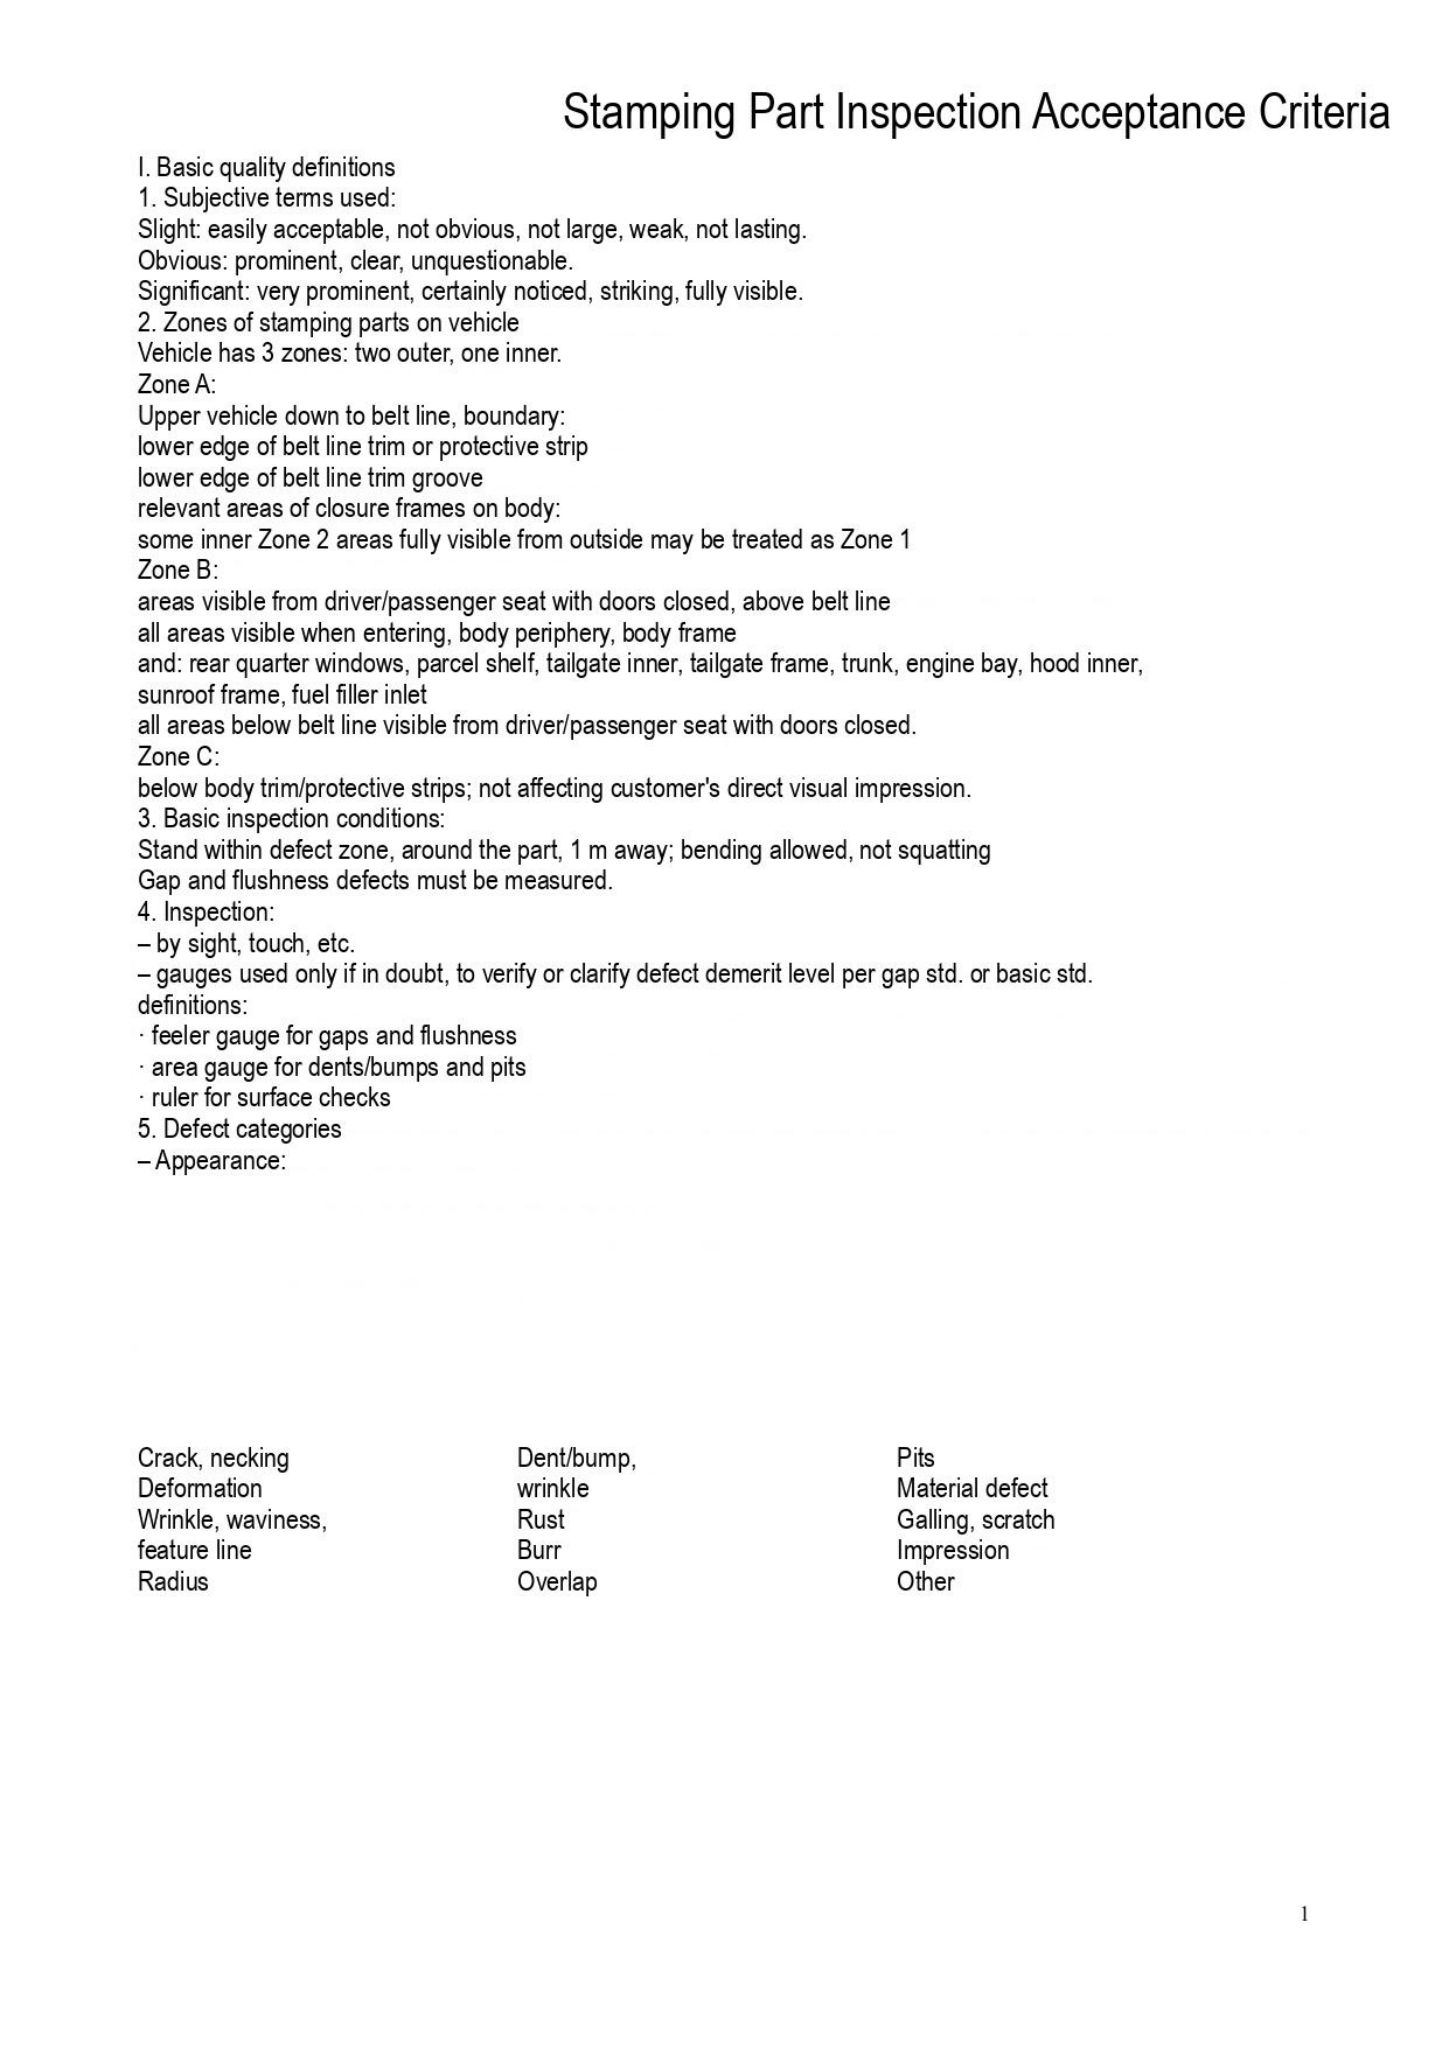Stamping Part Inspection Acceptance Criteria

I. Basic quality definitions
1. Subjective terms used:
Slight: easily acceptable, not obvious, not large, weak, not lasting.
Obvious: prominent, clear, unquestionable.
Significant: very prominent, certainly noticed, striking, fully visible.
2. Zones of stamping parts on vehicle
Vehicle has 3 zones: two outer, one inner.
Zone A:
Upper vehicle down to belt line, boundary:
lower edge of belt line trim or protective strip
lower edge of belt line trim groove
relevant areas of closure frames on body:
some inner Zone 2 areas fully visible from outside may be treated as Zone 1
Zone B:
areas visible from driver/passenger seat with doors closed, above belt line
all areas visible when entering, body periphery, body frame
and: rear quarter windows, parcel shelf, tailgate inner, tailgate frame, trunk, engine bay, hood inner, sunroof frame, fuel filler inlet
all areas below belt line visible from driver/passenger seat with doors closed.
Zone C:
below body trim/protective strips; not affecting customer's direct visual impression.
3. Basic inspection conditions:
Stand within defect zone, around the part, 1 m away; bending allowed, not squatting
Gap and flushness defects must be measured.
4. Inspection:
– by sight, touch, etc.
– gauges used only if in doubt, to verify or clarify defect demerit level per gap std. or basic std.
definitions:
· feeler gauge for gaps and flushness
· area gauge for dents/bumps and pits
· ruler for surface checks
5. Defect categories
– Appearance:

| | | |
|---|---|---|
| Crack, necking | Dent/bump, wrinkle | Pits |
| Deformation | Rust | Material defect |
| Wrinkle, waviness, feature line | Burr | Galling, scratch |
| Radius | Overlap | Impression |
| | | Other |

1
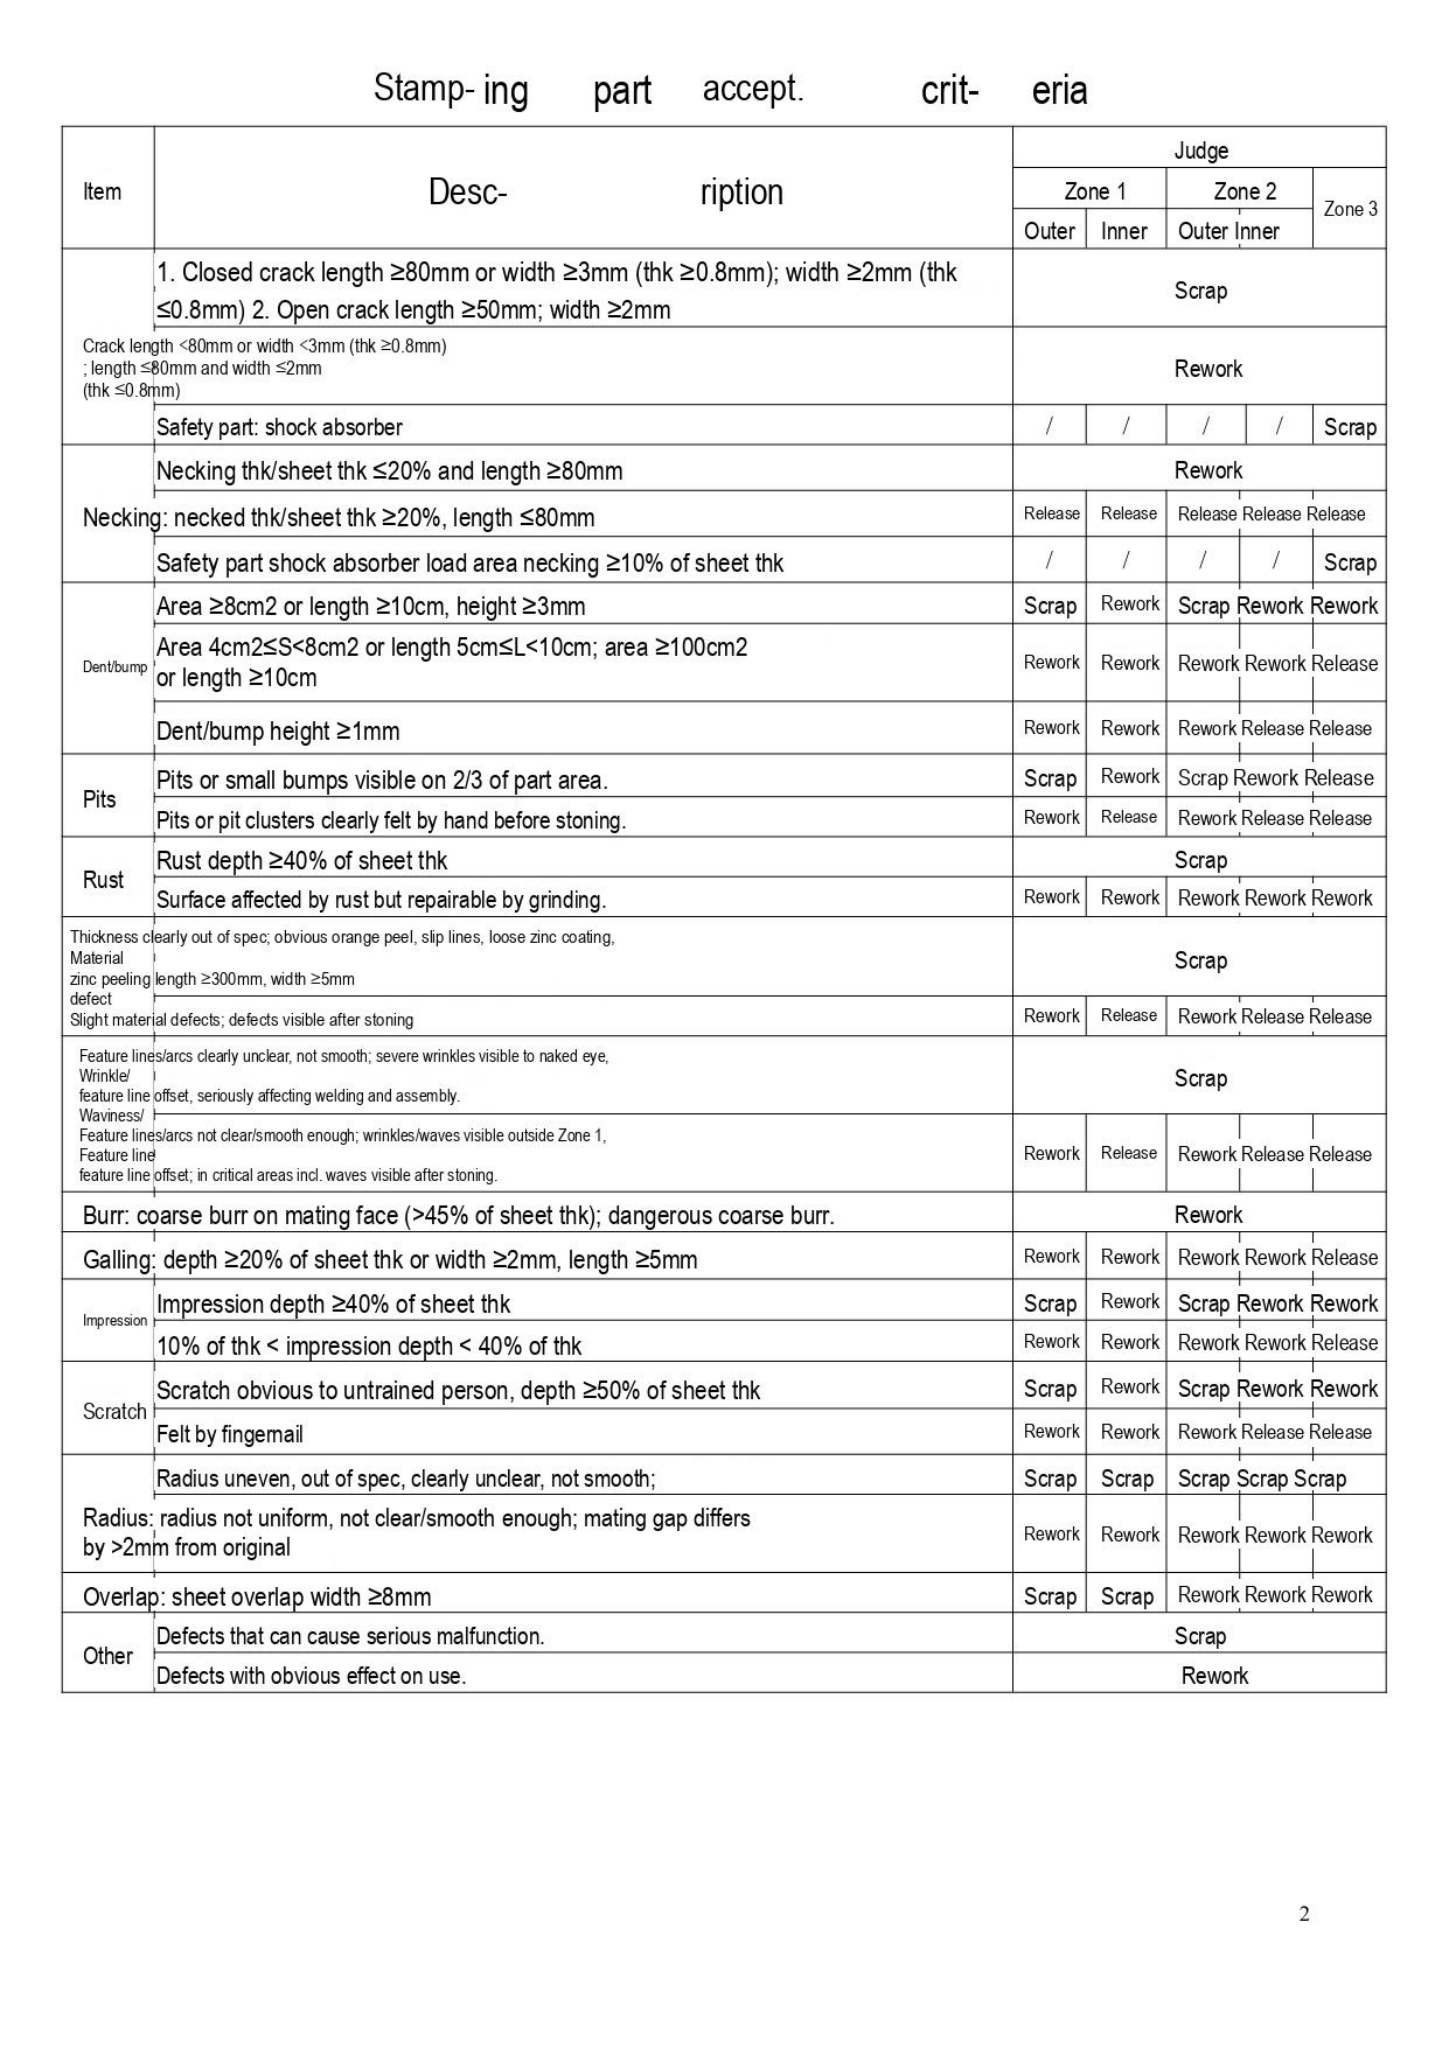Stamp- ing part accept. crit- eria

| Item | Description | Zone 1 Outer | Zone 1 Inner | Zone 2 Outer | Zone 2 Inner | Zone 3 |
|---|---|---|---|---|---|---|
| Crack | 1. Closed crack length ≥80mm or width ≥3mm (thk ≥0.8mm); width ≥2mm (thk ≤0.8mm) 2. Open crack length ≥50mm; width ≥2mm | Scrap | | | | |
| | Crack length <80mm or width <3mm (thk ≥0.8mm); length ≤80mm and width ≤2mm (thk ≤0.8mm) | Rework | | | | |
| | Safety part: shock absorber | / | / | / | / | Scrap |
| Necking | Necking thk/sheet thk ≤20% and length ≥80mm | Rework | | | | |
| | necked thk/sheet thk ≥20%, length ≤80mm | Release | Release | Release | Release | Release |
| | Safety part shock absorber load area necking ≥10% of sheet thk | / | / | / | / | Scrap |
| Dent/bump | Area ≥8cm2 or length ≥10cm, height ≥3mm | Scrap | Rework | Scrap | Rework | Rework |
| | Area 4cm2≤S<8cm2 or length 5cm≤L<10cm; area ≥100cm2 or length ≥10cm | Rework | Rework | Rework | Rework | Release |
| | Dent/bump height ≥1mm | Rework | Rework | Rework | Release | Release |
| Pits | Pits or small bumps visible on 2/3 of part area. | Scrap | Rework | Scrap | Rework | Release |
| | Pits or pit clusters clearly felt by hand before stoning. | Rework | Release | Rework | Release | Release |
| Rust | Rust depth ≥40% of sheet thk | Scrap | | | | |
| | Surface affected by rust but repairable by grinding. | Rework | Rework | Rework | Rework | Rework |
| Material defect | Thickness clearly out of spec; obvious orange peel, slip lines, loose zinc coating, zinc peeling length ≥300mm, width ≥5mm | Scrap | | | | |
| | Slight material defects; defects visible after stoning | Rework | Release | Rework | Release | Release |
| Wrinkle/ Waviness/ Feature line | Feature lines/arcs clearly unclear, not smooth; severe wrinkles visible to naked eye, feature line offset, seriously affecting welding and assembly. | Scrap | | | | |
| | Feature lines/arcs not clear/smooth enough; wrinkles/waves visible outside Zone 1, feature line offset; in critical areas incl. waves visible after stoning. | Rework | Release | Rework | Release | Release |
| Burr | coarse burr on mating face (>45% of sheet thk); dangerous coarse burr. | Rework | | | | |
| Galling | depth ≥20% of sheet thk or width ≥2mm, length ≥5mm | Rework | Rework | Rework | Rework | Release |
| Impression | Impression depth ≥40% of sheet thk | Scrap | Rework | Scrap | Rework | Rework |
| | 10% of thk < impression depth < 40% of thk | Rework | Rework | Rework | Rework | Release |
| Scratch | Scratch obvious to untrained person, depth ≥50% of sheet thk | Scrap | Rework | Scrap | Rework | Rework |
| | Felt by fingernail | Rework | Rework | Rework | Release | Release |
| Radius | Radius uneven, out of spec, clearly unclear, not smooth; | Scrap | Scrap | Scrap | Scrap | Scrap |
| | radius not uniform, not clear/smooth enough; mating gap differs by >2mm from original | Rework | Rework | Rework | Rework | Rework |
| Overlap | sheet overlap width ≥8mm | Scrap | Scrap | Rework | Rework | Rework |
| Other | Defects that can cause serious malfunction. | Scrap | | | | |
| | Defects with obvious effect on use. | Rework | | | | |

2
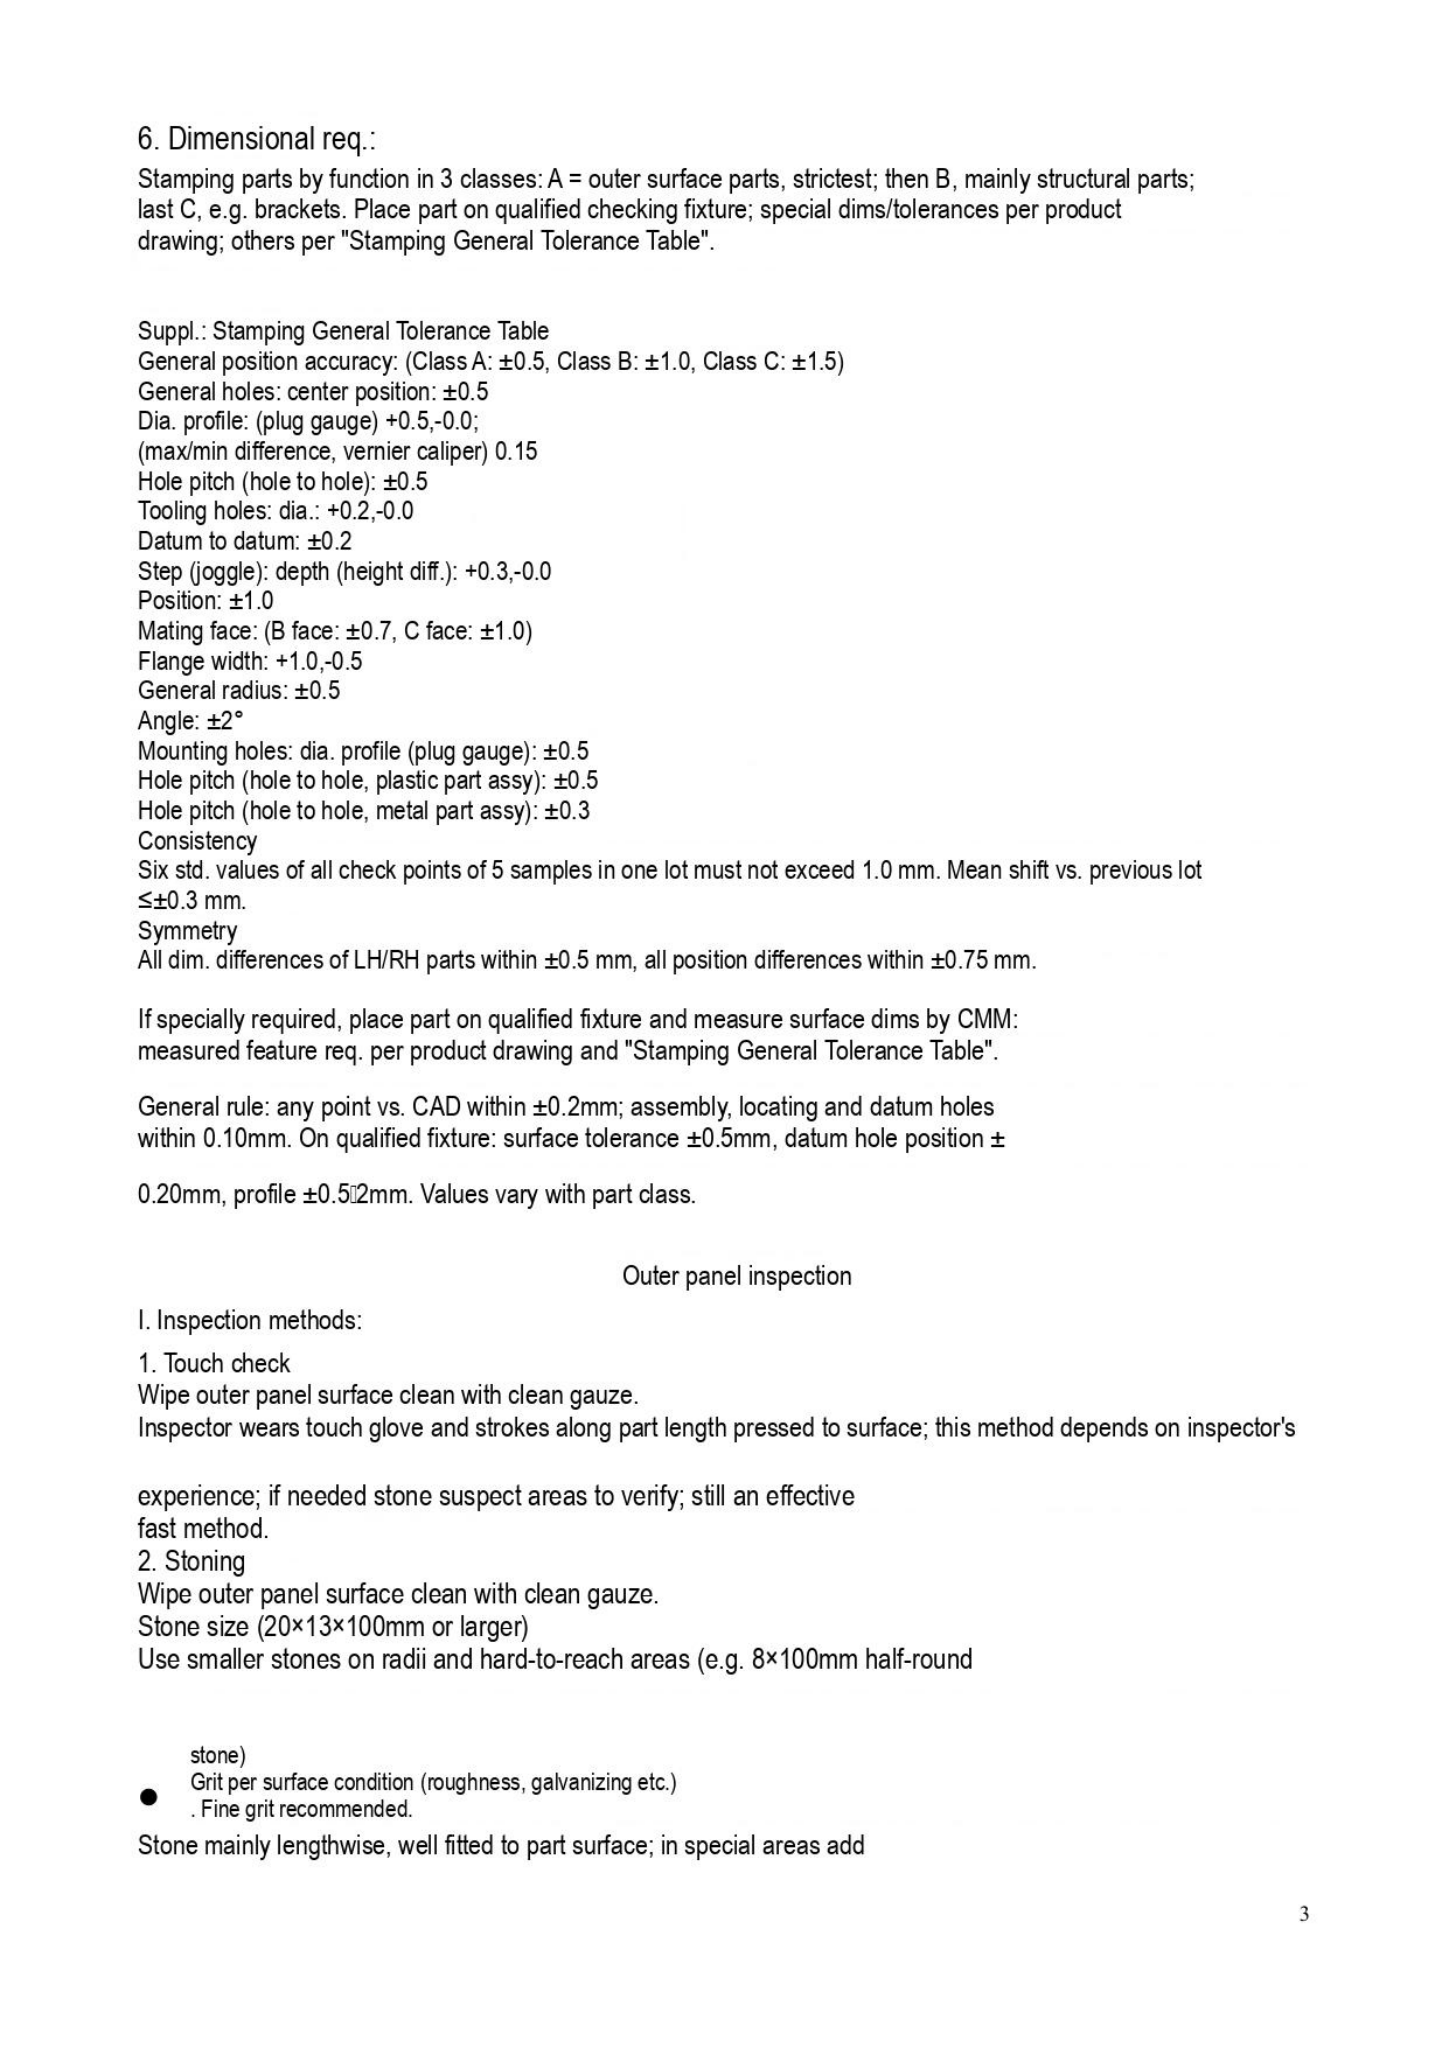6. Dimensional req.:
Stamping parts by function in 3 classes: A = outer surface parts, strictest; then B, mainly structural parts; last C, e.g. brackets. Place part on qualified checking fixture; special dims/tolerances per product drawing; others per "Stamping General Tolerance Table".

Suppl.: Stamping General Tolerance Table
General position accuracy: (Class A: ±0.5, Class B: ±1.0, Class C: ±1.5)
General holes: center position: ±0.5
Dia. profile: (plug gauge) +0.5,-0.0;
(max/min difference, vernier caliper) 0.15
Hole pitch (hole to hole): ±0.5
Tooling holes: dia.: +0.2,-0.0
Datum to datum: ±0.2
Step (joggle): depth (height diff.): +0.3,-0.0
Position: ±1.0
Mating face: (B face: ±0.7, C face: ±1.0)
Flange width: +1.0,-0.5
General radius: ±0.5
Angle: ±2°
Mounting holes: dia. profile (plug gauge): ±0.5
Hole pitch (hole to hole, plastic part assy): ±0.5
Hole pitch (hole to hole, metal part assy): ±0.3
Consistency
Six std. values of all check points of 5 samples in one lot must not exceed 1.0 mm. Mean shift vs. previous lot ≤±0.3 mm.
Symmetry
All dim. differences of LH/RH parts within ±0.5 mm, all position differences within ±0.75 mm.

If specially required, place part on qualified fixture and measure surface dims by CMM: measured feature req. per product drawing and "Stamping General Tolerance Table".

General rule: any point vs. CAD within ±0.2mm; assembly, locating and datum holes within 0.10mm. On qualified fixture: surface tolerance ±0.5mm, datum hole position ±

0.20mm, profile ±0.5 2mm. Values vary with part class.

Outer panel inspection

I. Inspection methods:

1. Touch check
Wipe outer panel surface clean with clean gauze.
Inspector wears touch glove and strokes along part length pressed to surface; this method depends on inspector's

experience; if needed stone suspect areas to verify; still an effective fast method.
2. Stoning
Wipe outer panel surface clean with clean gauze.
Stone size (20×13×100mm or larger)
Use smaller stones on radii and hard-to-reach areas (e.g. 8×100mm half-round

stone)
- Grit per surface condition (roughness, galvanizing etc.)
. Fine grit recommended.

Stone mainly lengthwise, well fitted to part surface; in special areas add

3
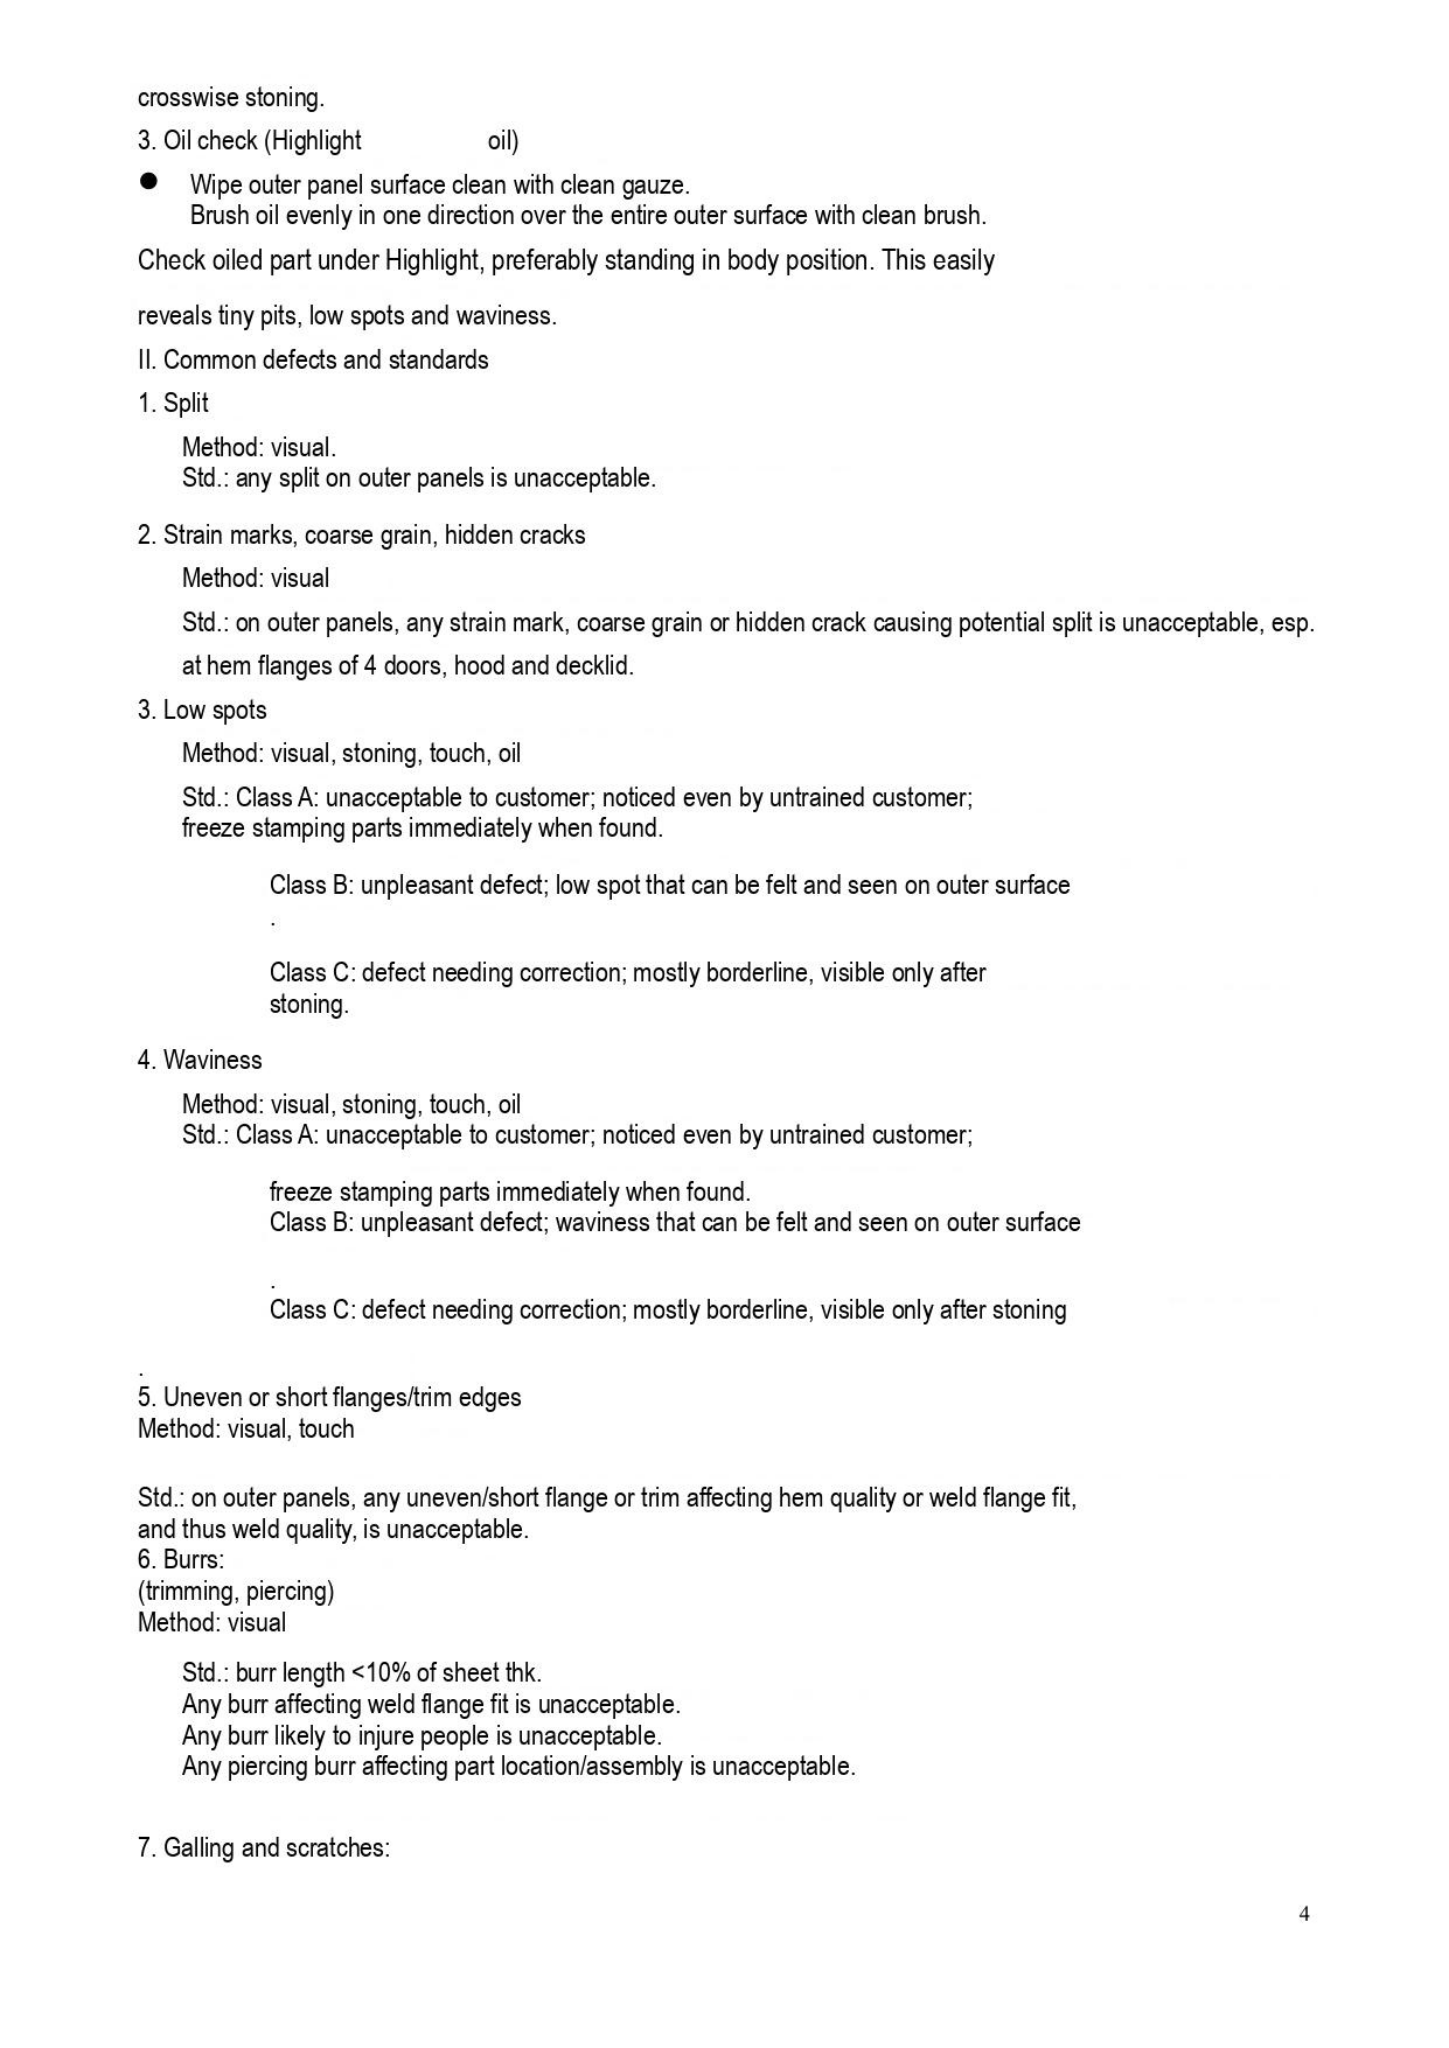crosswise stoning.

3. Oil check (Highlight oil)

● Wipe outer panel surface clean with clean gauze.
Brush oil evenly in one direction over the entire outer surface with clean brush.

Check oiled part under Highlight, preferably standing in body position. This easily

reveals tiny pits, low spots and waviness.

II. Common defects and standards

1. Split

Method: visual.
Std.: any split on outer panels is unacceptable.

2. Strain marks, coarse grain, hidden cracks

Method: visual

Std.: on outer panels, any strain mark, coarse grain or hidden crack causing potential split is unacceptable, esp. at hem flanges of 4 doors, hood and decklid.

3. Low spots

Method: visual, stoning, touch, oil

Std.: Class A: unacceptable to customer; noticed even by untrained customer; freeze stamping parts immediately when found.

Class B: unpleasant defect; low spot that can be felt and seen on outer surface
.

Class C: defect needing correction; mostly borderline, visible only after stoning.

4. Waviness

Method: visual, stoning, touch, oil
Std.: Class A: unacceptable to customer; noticed even by untrained customer;

freeze stamping parts immediately when found.
Class B: unpleasant defect; waviness that can be felt and seen on outer surface

.
Class C: defect needing correction; mostly borderline, visible only after stoning

.
5. Uneven or short flanges/trim edges
Method: visual, touch

Std.: on outer panels, any uneven/short flange or trim affecting hem quality or weld flange fit, and thus weld quality, is unacceptable.
6. Burrs:
(trimming, piercing)
Method: visual

Std.: burr length <10% of sheet thk.
Any burr affecting weld flange fit is unacceptable.
Any burr likely to injure people is unacceptable.
Any piercing burr affecting part location/assembly is unacceptable.

7. Galling and scratches:

4
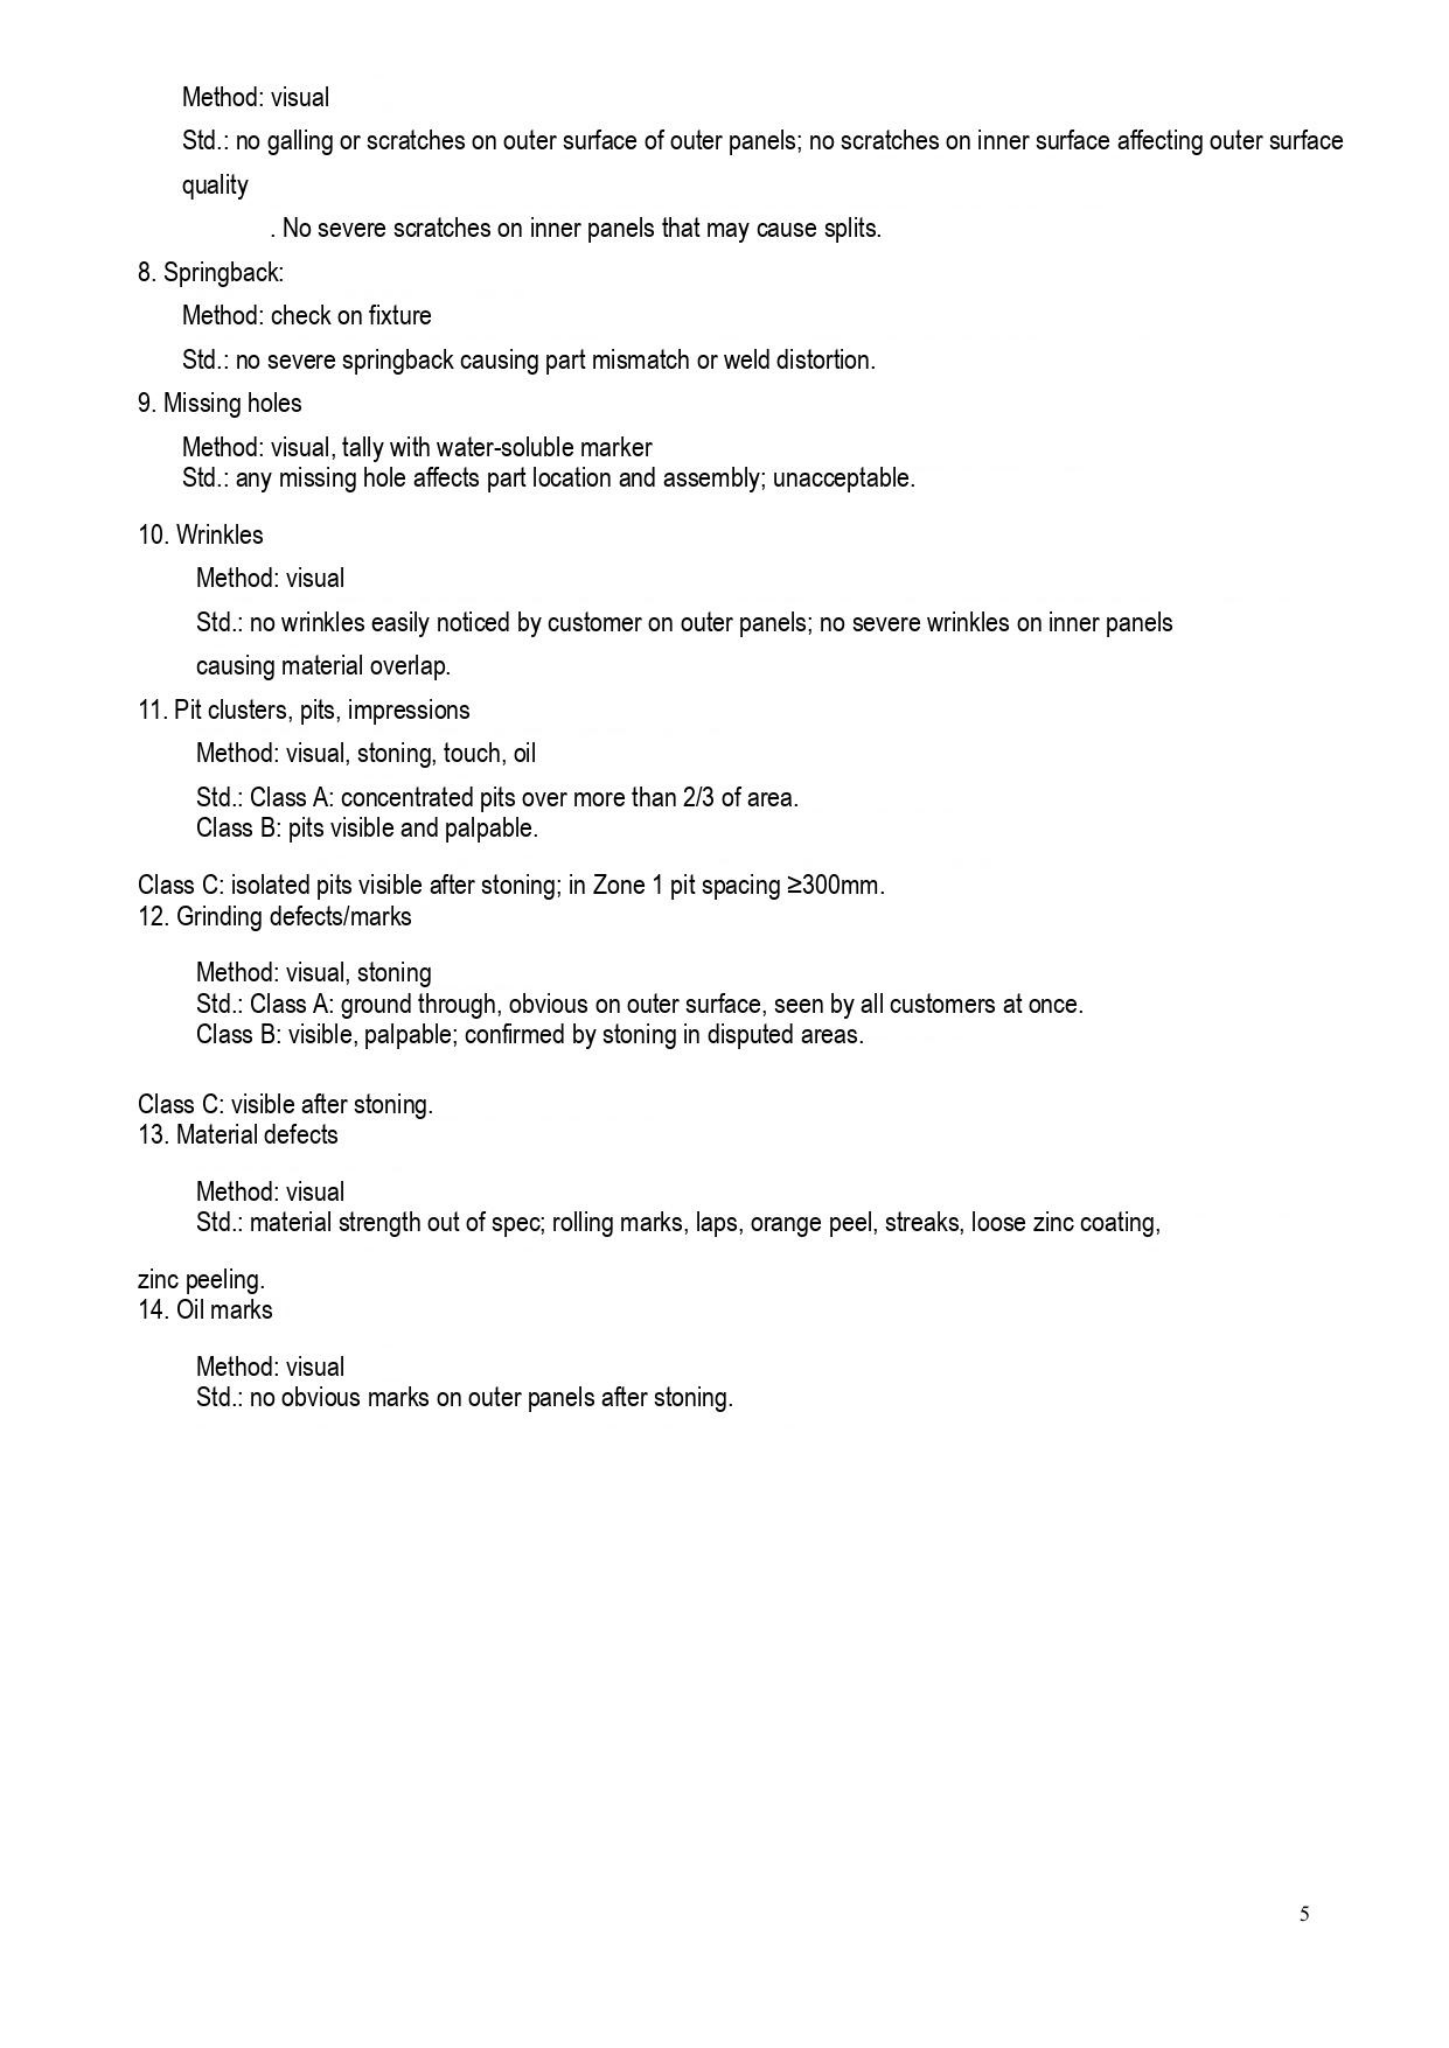Method: visual

Std.: no galling or scratches on outer surface of outer panels; no scratches on inner surface affecting outer surface quality

. No severe scratches on inner panels that may cause splits.

8. Springback:

Method: check on fixture

Std.: no severe springback causing part mismatch or weld distortion.

9. Missing holes

Method: visual, tally with water-soluble marker
Std.: any missing hole affects part location and assembly; unacceptable.

10. Wrinkles

Method: visual

Std.: no wrinkles easily noticed by customer on outer panels; no severe wrinkles on inner panels causing material overlap.

11. Pit clusters, pits, impressions

Method: visual, stoning, touch, oil

Std.: Class A: concentrated pits over more than 2/3 of area.
Class B: pits visible and palpable.

Class C: isolated pits visible after stoning; in Zone 1 pit spacing ≥300mm.
12. Grinding defects/marks

Method: visual, stoning
Std.: Class A: ground through, obvious on outer surface, seen by all customers at once.
Class B: visible, palpable; confirmed by stoning in disputed areas.

Class C: visible after stoning.
13. Material defects

Method: visual
Std.: material strength out of spec; rolling marks, laps, orange peel, streaks, loose zinc coating,

zinc peeling.
14. Oil marks

Method: visual
Std.: no obvious marks on outer panels after stoning.

5